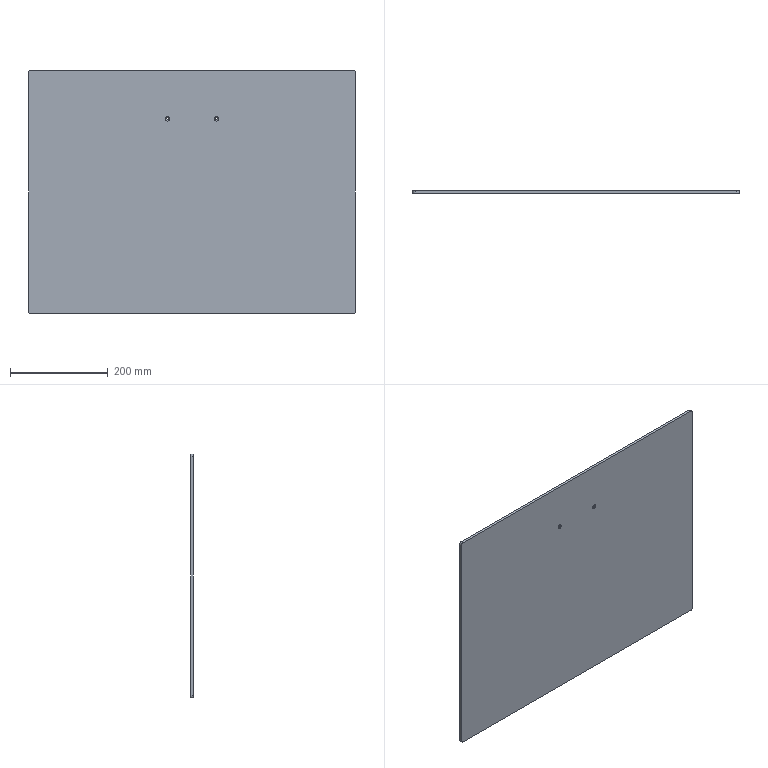Part | NX | features solid 2 | 1 solid | 18 faces | box 670 x 5 x 500 mm | volume 1674617 mm3 | cylinder 8 | plane 6 | cone 4 | commonest cylinder face diameters 5 x4 10 x4
STEP:
#1=CARTESIAN_POINT('',(1510.5,-650.,1045.));
#2=VERTEX_POINT('',#1);
#3=CARTESIAN_POINT('',(1512.5,-648.,1045.));
#4=VERTEX_POINT('',#3);
#5=CARTESIAN_POINT('',(1512.5,-648.,1045.));
#6=DIRECTION('',(-0.7071,-0.7071,0.));
#7=VECTOR('',#6,1000.);
#8=LINE('',#5,#7);
#9=EDGE_CURVE('',#2,#4,#8,.F.);
#10=ORIENTED_EDGE('',*,*,#9,.T.);
#11=CARTESIAN_POINT('',(1517.5,-648.,1045.));
#12=VERTEX_POINT('',#11);
#13=CARTESIAN_POINT('',(1515.,-648.,1045.));
#14=DIRECTION('',(0.,-1.,0.));
#15=DIRECTION('',(1.,0.,0.));
#16=AXIS2_PLACEMENT_3D('',#13,#14,#15);
#17=CIRCLE('',#16,2.5);
#18=EDGE_CURVE('',#12,#4,#17,.T.);
#19=ORIENTED_EDGE('',*,*,#18,.F.);
#20=CARTESIAN_POINT('',(1519.5,-650.,1045.));
#21=VERTEX_POINT('',#20);
#22=CARTESIAN_POINT('',(1517.5,-648.,1045.));
#23=DIRECTION('',(0.7071,-0.7071,0.));
#24=VECTOR('',#23,1000.);
#25=LINE('',#22,#24);
#26=EDGE_CURVE('',#12,#21,#25,.T.);
#27=ORIENTED_EDGE('',*,*,#26,.T.);
#28=CARTESIAN_POINT('',(1515.,-650.,1045.));
#29=DIRECTION('',(0.,1.,0.));
#30=DIRECTION('',(1.,0.,0.));
#31=AXIS2_PLACEMENT_3D('',#28,#29,#30);
#32=CIRCLE('',#31,4.5);
#33=EDGE_CURVE('',#2,#21,#32,.T.);
#34=ORIENTED_EDGE('',*,*,#33,.F.);
#35=EDGE_LOOP('',(#10,#19,#27,#34));
#36=FACE_BOUND('',#35,.T.);
#37=CARTESIAN_POINT('',(1515.,-648.,1045.));
#38=DIRECTION('',(0.,-1.,0.));
#39=DIRECTION('',(1.,0.,0.));
#40=AXIS2_PLACEMENT_3D('',#37,#38,#39);
#41=CONICAL_SURFACE('',#40,2.5,0.7854);
#42=ADVANCED_FACE('',(#36),#41,.F.);
#43=CARTESIAN_POINT('',(1610.5,-650.,1045.));
#44=VERTEX_POINT('',#43);
#45=CARTESIAN_POINT('',(1612.5,-648.,1045.));
#46=VERTEX_POINT('',#45);
#47=CARTESIAN_POINT('',(1612.5,-648.,1045.));
#48=DIRECTION('',(-0.7071,-0.7071,0.));
#49=VECTOR('',#48,1000.);
#50=LINE('',#47,#49);
#51=EDGE_CURVE('',#44,#46,#50,.F.);
#52=ORIENTED_EDGE('',*,*,#51,.T.);
#53=CARTESIAN_POINT('',(1617.5,-648.,1045.));
#54=VERTEX_POINT('',#53);
#55=CARTESIAN_POINT('',(1615.,-648.,1045.));
#56=DIRECTION('',(0.,-1.,0.));
#57=DIRECTION('',(1.,0.,0.));
#58=AXIS2_PLACEMENT_3D('',#55,#56,#57);
#59=CIRCLE('',#58,2.5);
#60=EDGE_CURVE('',#54,#46,#59,.T.);
#61=ORIENTED_EDGE('',*,*,#60,.F.);
#62=CARTESIAN_POINT('',(1619.5,-650.,1045.));
#63=VERTEX_POINT('',#62);
#64=CARTESIAN_POINT('',(1617.5,-648.,1045.));
#65=DIRECTION('',(0.7071,-0.7071,0.));
#66=VECTOR('',#65,1000.);
#67=LINE('',#64,#66);
#68=EDGE_CURVE('',#54,#63,#67,.T.);
#69=ORIENTED_EDGE('',*,*,#68,.T.);
#70=CARTESIAN_POINT('',(1615.,-650.,1045.));
#71=DIRECTION('',(0.,1.,0.));
#72=DIRECTION('',(1.,0.,0.));
#73=AXIS2_PLACEMENT_3D('',#70,#71,#72);
#74=CIRCLE('',#73,4.5);
#75=EDGE_CURVE('',#44,#63,#74,.T.);
#76=ORIENTED_EDGE('',*,*,#75,.F.);
#77=EDGE_LOOP('',(#52,#61,#69,#76));
#78=FACE_BOUND('',#77,.T.);
#79=CARTESIAN_POINT('',(1615.,-648.,1045.));
#80=DIRECTION('',(0.,-1.,0.));
#81=DIRECTION('',(1.,0.,0.));
#82=AXIS2_PLACEMENT_3D('',#79,#80,#81);
#83=CONICAL_SURFACE('',#82,2.5,0.7854);
#84=ADVANCED_FACE('',(#78),#83,.F.);
#85=CARTESIAN_POINT('',(1517.5,-645.,1045.));
#86=VERTEX_POINT('',#85);
#87=CARTESIAN_POINT('',(1517.5,-1481.017,1045.));
#88=DIRECTION('',(0.,1.,0.));
#89=VECTOR('',#88,1000.);
#90=LINE('',#87,#89);
#91=EDGE_CURVE('',#86,#12,#90,.F.);
#92=ORIENTED_EDGE('',*,*,#91,.T.);
#93=ORIENTED_EDGE('',*,*,#18,.T.);
#94=CARTESIAN_POINT('',(1512.5,-645.,1045.));
#95=VERTEX_POINT('',#94);
#96=CARTESIAN_POINT('',(1512.5,-1481.017,1045.));
#97=DIRECTION('',(0.,1.,0.));
#98=VECTOR('',#97,1000.);
#99=LINE('',#96,#98);
#100=EDGE_CURVE('',#4,#95,#99,.T.);
#101=ORIENTED_EDGE('',*,*,#100,.T.);
#102=CARTESIAN_POINT('',(1515.,-645.,1045.));
#103=DIRECTION('',(0.,1.,0.));
#104=DIRECTION('',(-1.,0.,0.));
#105=AXIS2_PLACEMENT_3D('',#102,#103,#104);
#106=CIRCLE('',#105,2.5);
#107=EDGE_CURVE('',#95,#86,#106,.T.);
#108=ORIENTED_EDGE('',*,*,#107,.T.);
#109=EDGE_LOOP('',(#92,#93,#101,#108));
#110=FACE_BOUND('',#109,.T.);
#111=CARTESIAN_POINT('',(1515.,-1481.017,1045.));
#112=DIRECTION('',(0.,1.,0.));
#113=DIRECTION('',(-1.,0.,0.));
#114=AXIS2_PLACEMENT_3D('',#111,#112,#113);
#115=CYLINDRICAL_SURFACE('',#114,2.5);
#116=ADVANCED_FACE('',(#110),#115,.F.);
#117=CARTESIAN_POINT('',(1617.5,-645.,1045.));
#118=VERTEX_POINT('',#117);
#119=CARTESIAN_POINT('',(1617.5,-1481.017,1045.));
#120=DIRECTION('',(0.,1.,0.));
#121=VECTOR('',#120,1000.);
#122=LINE('',#119,#121);
#123=EDGE_CURVE('',#118,#54,#122,.F.);
#124=ORIENTED_EDGE('',*,*,#123,.T.);
#125=ORIENTED_EDGE('',*,*,#60,.T.);
#126=CARTESIAN_POINT('',(1612.5,-645.,1045.));
#127=VERTEX_POINT('',#126);
#128=CARTESIAN_POINT('',(1612.5,-1481.017,1045.));
#129=DIRECTION('',(0.,1.,0.));
#130=VECTOR('',#129,1000.);
#131=LINE('',#128,#130);
#132=EDGE_CURVE('',#46,#127,#131,.T.);
#133=ORIENTED_EDGE('',*,*,#132,.T.);
#134=CARTESIAN_POINT('',(1615.,-645.,1045.));
#135=DIRECTION('',(0.,1.,0.));
#136=DIRECTION('',(-1.,0.,0.));
#137=AXIS2_PLACEMENT_3D('',#134,#135,#136);
#138=CIRCLE('',#137,2.5);
#139=EDGE_CURVE('',#127,#118,#138,.T.);
#140=ORIENTED_EDGE('',*,*,#139,.T.);
#141=EDGE_LOOP('',(#124,#125,#133,#140));
#142=FACE_BOUND('',#141,.T.);
#143=CARTESIAN_POINT('',(1615.,-1481.017,1045.));
#144=DIRECTION('',(0.,1.,0.));
#145=DIRECTION('',(-1.,0.,0.));
#146=AXIS2_PLACEMENT_3D('',#143,#144,#145);
#147=CYLINDRICAL_SURFACE('',#146,2.5);
#148=ADVANCED_FACE('',(#142),#147,.F.);
#149=CARTESIAN_POINT('',(1235.,-645.,645.));
#150=VERTEX_POINT('',#149);
#151=CARTESIAN_POINT('',(1230.,-645.,650.));
#152=VERTEX_POINT('',#151);
#153=CARTESIAN_POINT('',(1235.,-645.,650.));
#154=DIRECTION('',(0.,1.,0.));
#155=DIRECTION('',(1.,0.,0.));
#156=AXIS2_PLACEMENT_3D('',#153,#154,#155);
#157=CIRCLE('',#156,5.);
#158=EDGE_CURVE('',#150,#152,#157,.T.);
#159=ORIENTED_EDGE('',*,*,#158,.F.);
#160=CARTESIAN_POINT('',(1235.,-650.,645.));
#161=VERTEX_POINT('',#160);
#162=CARTESIAN_POINT('',(1235.,-645.,645.));
#163=DIRECTION('',(0.,1.,0.));
#164=VECTOR('',#163,1000.);
#165=LINE('',#162,#164);
#166=EDGE_CURVE('',#161,#150,#165,.T.);
#167=ORIENTED_EDGE('',*,*,#166,.F.);
#168=CARTESIAN_POINT('',(1230.,-650.,650.));
#169=VERTEX_POINT('',#168);
#170=CARTESIAN_POINT('',(1235.,-650.,650.));
#171=DIRECTION('',(0.,-1.,0.));
#172=DIRECTION('',(1.,0.,0.));
#173=AXIS2_PLACEMENT_3D('',#170,#171,#172);
#174=CIRCLE('',#173,5.);
#175=EDGE_CURVE('',#169,#161,#174,.T.);
#176=ORIENTED_EDGE('',*,*,#175,.F.);
#177=CARTESIAN_POINT('',(1230.,-645.,650.));
#178=DIRECTION('',(0.,-1.,0.));
#179=VECTOR('',#178,1000.);
#180=LINE('',#177,#179);
#181=EDGE_CURVE('',#152,#169,#180,.T.);
#182=ORIENTED_EDGE('',*,*,#181,.F.);
#183=EDGE_LOOP('',(#159,#167,#176,#182));
#184=FACE_BOUND('',#183,.T.);
#185=CARTESIAN_POINT('',(1235.,-645.,650.));
#186=DIRECTION('',(0.,-1.,0.));
#187=DIRECTION('',(1.,0.,0.));
#188=AXIS2_PLACEMENT_3D('',#185,#186,#187);
#189=CYLINDRICAL_SURFACE('',#188,5.);
#190=ADVANCED_FACE('',(#184),#189,.T.);
#191=CARTESIAN_POINT('',(1230.,-645.,1140.));
#192=VERTEX_POINT('',#191);
#193=CARTESIAN_POINT('',(1235.,-645.,1145.));
#194=VERTEX_POINT('',#193);
#195=CARTESIAN_POINT('',(1235.,-645.,1140.));
#196=DIRECTION('',(0.,1.,0.));
#197=DIRECTION('',(1.,0.,0.));
#198=AXIS2_PLACEMENT_3D('',#195,#196,#197);
#199=CIRCLE('',#198,5.);
#200=EDGE_CURVE('',#192,#194,#199,.T.);
#201=ORIENTED_EDGE('',*,*,#200,.F.);
#202=CARTESIAN_POINT('',(1230.,-650.,1140.));
#203=VERTEX_POINT('',#202);
#204=CARTESIAN_POINT('',(1230.,-645.,1140.));
#205=DIRECTION('',(0.,1.,0.));
#206=VECTOR('',#205,1000.);
#207=LINE('',#204,#206);
#208=EDGE_CURVE('',#203,#192,#207,.T.);
#209=ORIENTED_EDGE('',*,*,#208,.F.);
#210=CARTESIAN_POINT('',(1235.,-650.,1145.));
#211=VERTEX_POINT('',#210);
#212=CARTESIAN_POINT('',(1235.,-650.,1140.));
#213=DIRECTION('',(0.,-1.,0.));
#214=DIRECTION('',(1.,0.,0.));
#215=AXIS2_PLACEMENT_3D('',#212,#213,#214);
#216=CIRCLE('',#215,5.);
#217=EDGE_CURVE('',#211,#203,#216,.T.);
#218=ORIENTED_EDGE('',*,*,#217,.F.);
#219=CARTESIAN_POINT('',(1235.,-645.,1145.));
#220=DIRECTION('',(0.,-1.,0.));
#221=VECTOR('',#220,1000.);
#222=LINE('',#219,#221);
#223=EDGE_CURVE('',#194,#211,#222,.T.);
#224=ORIENTED_EDGE('',*,*,#223,.F.);
#225=EDGE_LOOP('',(#201,#209,#218,#224));
#226=FACE_BOUND('',#225,.T.);
#227=CARTESIAN_POINT('',(1235.,-645.,1140.));
#228=DIRECTION('',(0.,-1.,0.));
#229=DIRECTION('',(1.,0.,0.));
#230=AXIS2_PLACEMENT_3D('',#227,#228,#229);
#231=CYLINDRICAL_SURFACE('',#230,5.);
#232=ADVANCED_FACE('',(#226),#231,.T.);
#233=CARTESIAN_POINT('',(1895.,-645.,1145.));
#234=VERTEX_POINT('',#233);
#235=CARTESIAN_POINT('',(1900.,-645.,1140.));
#236=VERTEX_POINT('',#235);
#237=CARTESIAN_POINT('',(1895.,-645.,1140.));
#238=DIRECTION('',(0.,1.,0.));
#239=DIRECTION('',(1.,0.,0.));
#240=AXIS2_PLACEMENT_3D('',#237,#238,#239);
#241=CIRCLE('',#240,5.);
#242=EDGE_CURVE('',#234,#236,#241,.T.);
#243=ORIENTED_EDGE('',*,*,#242,.F.);
#244=CARTESIAN_POINT('',(1895.,-650.,1145.));
#245=VERTEX_POINT('',#244);
#246=CARTESIAN_POINT('',(1895.,-645.,1145.));
#247=DIRECTION('',(0.,1.,0.));
#248=VECTOR('',#247,1000.);
#249=LINE('',#246,#248);
#250=EDGE_CURVE('',#245,#234,#249,.T.);
#251=ORIENTED_EDGE('',*,*,#250,.F.);
#252=CARTESIAN_POINT('',(1900.,-650.,1140.));
#253=VERTEX_POINT('',#252);
#254=CARTESIAN_POINT('',(1895.,-650.,1140.));
#255=DIRECTION('',(0.,-1.,0.));
#256=DIRECTION('',(1.,0.,0.));
#257=AXIS2_PLACEMENT_3D('',#254,#255,#256);
#258=CIRCLE('',#257,5.);
#259=EDGE_CURVE('',#253,#245,#258,.T.);
#260=ORIENTED_EDGE('',*,*,#259,.F.);
#261=CARTESIAN_POINT('',(1900.,-645.,1140.));
#262=DIRECTION('',(0.,-1.,0.));
#263=VECTOR('',#262,1000.);
#264=LINE('',#261,#263);
#265=EDGE_CURVE('',#236,#253,#264,.T.);
#266=ORIENTED_EDGE('',*,*,#265,.F.);
#267=EDGE_LOOP('',(#243,#251,#260,#266));
#268=FACE_BOUND('',#267,.T.);
#269=CARTESIAN_POINT('',(1895.,-645.,1140.));
#270=DIRECTION('',(0.,-1.,0.));
#271=DIRECTION('',(1.,0.,0.));
#272=AXIS2_PLACEMENT_3D('',#269,#270,#271);
#273=CYLINDRICAL_SURFACE('',#272,5.);
#274=ADVANCED_FACE('',(#268),#273,.T.);
#275=CARTESIAN_POINT('',(1900.,-645.,650.));
#276=VERTEX_POINT('',#275);
#277=CARTESIAN_POINT('',(1895.,-645.,645.));
#278=VERTEX_POINT('',#277);
#279=CARTESIAN_POINT('',(1895.,-645.,650.));
#280=DIRECTION('',(0.,1.,0.));
#281=DIRECTION('',(1.,0.,0.));
#282=AXIS2_PLACEMENT_3D('',#279,#280,#281);
#283=CIRCLE('',#282,5.);
#284=EDGE_CURVE('',#276,#278,#283,.T.);
#285=ORIENTED_EDGE('',*,*,#284,.F.);
#286=CARTESIAN_POINT('',(1900.,-650.,650.));
#287=VERTEX_POINT('',#286);
#288=CARTESIAN_POINT('',(1900.,-645.,650.));
#289=DIRECTION('',(0.,1.,0.));
#290=VECTOR('',#289,1000.);
#291=LINE('',#288,#290);
#292=EDGE_CURVE('',#287,#276,#291,.T.);
#293=ORIENTED_EDGE('',*,*,#292,.F.);
#294=CARTESIAN_POINT('',(1895.,-650.,645.));
#295=VERTEX_POINT('',#294);
#296=CARTESIAN_POINT('',(1895.,-650.,650.));
#297=DIRECTION('',(0.,-1.,0.));
#298=DIRECTION('',(1.,0.,0.));
#299=AXIS2_PLACEMENT_3D('',#296,#297,#298);
#300=CIRCLE('',#299,5.);
#301=EDGE_CURVE('',#295,#287,#300,.T.);
#302=ORIENTED_EDGE('',*,*,#301,.F.);
#303=CARTESIAN_POINT('',(1895.,-645.,645.));
#304=DIRECTION('',(0.,-1.,0.));
#305=VECTOR('',#304,1000.);
#306=LINE('',#303,#305);
#307=EDGE_CURVE('',#278,#295,#306,.T.);
#308=ORIENTED_EDGE('',*,*,#307,.F.);
#309=EDGE_LOOP('',(#285,#293,#302,#308));
#310=FACE_BOUND('',#309,.T.);
#311=CARTESIAN_POINT('',(1895.,-645.,650.));
#312=DIRECTION('',(0.,-1.,0.));
#313=DIRECTION('',(1.,0.,0.));
#314=AXIS2_PLACEMENT_3D('',#311,#312,#313);
#315=CYLINDRICAL_SURFACE('',#314,5.);
#316=ADVANCED_FACE('',(#310),#315,.T.);
#317=CARTESIAN_POINT('',(1515.,-650.,1045.));
#318=DIRECTION('',(0.,1.,0.));
#319=DIRECTION('',(1.,0.,0.));
#320=AXIS2_PLACEMENT_3D('',#317,#318,#319);
#321=CIRCLE('',#320,4.5);
#322=EDGE_CURVE('',#21,#2,#321,.T.);
#323=ORIENTED_EDGE('',*,*,#322,.T.);
#324=ORIENTED_EDGE('',*,*,#33,.T.);
#325=EDGE_LOOP('',(#323,#324));
#326=FACE_BOUND('',#325,.T.);
#327=CARTESIAN_POINT('',(1615.,-650.,1045.));
#328=DIRECTION('',(0.,1.,0.));
#329=DIRECTION('',(1.,0.,0.));
#330=AXIS2_PLACEMENT_3D('',#327,#328,#329);
#331=CIRCLE('',#330,4.5);
#332=EDGE_CURVE('',#63,#44,#331,.T.);
#333=ORIENTED_EDGE('',*,*,#332,.T.);
#334=ORIENTED_EDGE('',*,*,#75,.T.);
#335=EDGE_LOOP('',(#333,#334));
#336=FACE_BOUND('',#335,.T.);
#337=CARTESIAN_POINT('',(1230.,-650.,1145.));
#338=DIRECTION('',(0.,0.,-1.));
#339=VECTOR('',#338,1000.);
#340=LINE('',#337,#339);
#341=EDGE_CURVE('',#203,#169,#340,.T.);
#342=ORIENTED_EDGE('',*,*,#341,.T.);
#343=ORIENTED_EDGE('',*,*,#175,.T.);
#344=CARTESIAN_POINT('',(1230.,-650.,645.));
#345=DIRECTION('',(1.,0.,0.));
#346=VECTOR('',#345,1000.);
#347=LINE('',#344,#346);
#348=EDGE_CURVE('',#161,#295,#347,.T.);
#349=ORIENTED_EDGE('',*,*,#348,.T.);
#350=ORIENTED_EDGE('',*,*,#301,.T.);
#351=CARTESIAN_POINT('',(1900.,-650.,645.));
#352=DIRECTION('',(0.,0.,1.));
#353=VECTOR('',#352,1000.);
#354=LINE('',#351,#353);
#355=EDGE_CURVE('',#287,#253,#354,.T.);
#356=ORIENTED_EDGE('',*,*,#355,.T.);
#357=ORIENTED_EDGE('',*,*,#259,.T.);
#358=CARTESIAN_POINT('',(1900.,-650.,1145.));
#359=DIRECTION('',(-1.,0.,0.));
#360=VECTOR('',#359,1000.);
#361=LINE('',#358,#360);
#362=EDGE_CURVE('',#245,#211,#361,.T.);
#363=ORIENTED_EDGE('',*,*,#362,.T.);
#364=ORIENTED_EDGE('',*,*,#217,.T.);
#365=EDGE_LOOP('',(#342,#343,#349,#350,#356,#357,#363,#364));
#366=FACE_BOUND('',#365,.T.);
#367=CARTESIAN_POINT('',(1565.,-650.,895.));
#368=DIRECTION('',(0.,-1.,0.));
#369=DIRECTION('',(-1.,0.,0.));
#370=AXIS2_PLACEMENT_3D('',#367,#368,#369);
#371=PLANE('',#370);
#372=ADVANCED_FACE('',(#326,#336,#366),#371,.T.);
#373=ORIENTED_EDGE('',*,*,#139,.F.);
#374=CARTESIAN_POINT('',(1615.,-645.,1045.));
#375=DIRECTION('',(0.,1.,0.));
#376=DIRECTION('',(-1.,0.,0.));
#377=AXIS2_PLACEMENT_3D('',#374,#375,#376);
#378=CIRCLE('',#377,2.5);
#379=EDGE_CURVE('',#118,#127,#378,.T.);
#380=ORIENTED_EDGE('',*,*,#379,.F.);
#381=EDGE_LOOP('',(#373,#380));
#382=FACE_BOUND('',#381,.T.);
#383=ORIENTED_EDGE('',*,*,#107,.F.);
#384=CARTESIAN_POINT('',(1515.,-645.,1045.));
#385=DIRECTION('',(0.,1.,0.));
#386=DIRECTION('',(-1.,0.,0.));
#387=AXIS2_PLACEMENT_3D('',#384,#385,#386);
#388=CIRCLE('',#387,2.5);
#389=EDGE_CURVE('',#86,#95,#388,.T.);
#390=ORIENTED_EDGE('',*,*,#389,.F.);
#391=EDGE_LOOP('',(#383,#390));
#392=FACE_BOUND('',#391,.T.);
#393=CARTESIAN_POINT('',(1230.,-645.,645.));
#394=DIRECTION('',(1.,0.,0.));
#395=VECTOR('',#394,1000.);
#396=LINE('',#393,#395);
#397=EDGE_CURVE('',#150,#278,#396,.T.);
#398=ORIENTED_EDGE('',*,*,#397,.F.);
#399=ORIENTED_EDGE('',*,*,#158,.T.);
#400=CARTESIAN_POINT('',(1230.,-645.,1145.));
#401=DIRECTION('',(0.,0.,-1.));
#402=VECTOR('',#401,1000.);
#403=LINE('',#400,#402);
#404=EDGE_CURVE('',#192,#152,#403,.T.);
#405=ORIENTED_EDGE('',*,*,#404,.F.);
#406=ORIENTED_EDGE('',*,*,#200,.T.);
#407=CARTESIAN_POINT('',(1900.,-645.,1145.));
#408=DIRECTION('',(-1.,0.,0.));
#409=VECTOR('',#408,1000.);
#410=LINE('',#407,#409);
#411=EDGE_CURVE('',#234,#194,#410,.T.);
#412=ORIENTED_EDGE('',*,*,#411,.F.);
#413=ORIENTED_EDGE('',*,*,#242,.T.);
#414=CARTESIAN_POINT('',(1900.,-645.,645.));
#415=DIRECTION('',(0.,0.,1.));
#416=VECTOR('',#415,1000.);
#417=LINE('',#414,#416);
#418=EDGE_CURVE('',#276,#236,#417,.T.);
#419=ORIENTED_EDGE('',*,*,#418,.F.);
#420=ORIENTED_EDGE('',*,*,#284,.T.);
#421=EDGE_LOOP('',(#398,#399,#405,#406,#412,#413,#419,#420));
#422=FACE_BOUND('',#421,.T.);
#423=CARTESIAN_POINT('',(1565.,-645.,895.));
#424=DIRECTION('',(0.,-1.,0.));
#425=DIRECTION('',(-1.,0.,0.));
#426=AXIS2_PLACEMENT_3D('',#423,#424,#425);
#427=PLANE('',#426);
#428=ADVANCED_FACE('',(#382,#392,#422),#427,.F.);
#429=ORIENTED_EDGE('',*,*,#411,.T.);
#430=ORIENTED_EDGE('',*,*,#223,.T.);
#431=ORIENTED_EDGE('',*,*,#362,.F.);
#432=ORIENTED_EDGE('',*,*,#250,.T.);
#433=EDGE_LOOP('',(#429,#430,#431,#432));
#434=FACE_BOUND('',#433,.T.);
#435=CARTESIAN_POINT('',(1900.,-645.,1145.));
#436=DIRECTION('',(0.,0.,1.));
#437=DIRECTION('',(1.,0.,0.));
#438=AXIS2_PLACEMENT_3D('',#435,#436,#437);
#439=PLANE('',#438);
#440=ADVANCED_FACE('',(#434),#439,.T.);
#441=ORIENTED_EDGE('',*,*,#418,.T.);
#442=ORIENTED_EDGE('',*,*,#265,.T.);
#443=ORIENTED_EDGE('',*,*,#355,.F.);
#444=ORIENTED_EDGE('',*,*,#292,.T.);
#445=EDGE_LOOP('',(#441,#442,#443,#444));
#446=FACE_BOUND('',#445,.T.);
#447=CARTESIAN_POINT('',(1900.,-645.,645.));
#448=DIRECTION('',(1.,0.,0.));
#449=DIRECTION('',(0.,0.,1.));
#450=AXIS2_PLACEMENT_3D('',#447,#448,#449);
#451=PLANE('',#450);
#452=ADVANCED_FACE('',(#446),#451,.T.);
#453=ORIENTED_EDGE('',*,*,#348,.F.);
#454=ORIENTED_EDGE('',*,*,#166,.T.);
#455=ORIENTED_EDGE('',*,*,#397,.T.);
#456=ORIENTED_EDGE('',*,*,#307,.T.);
#457=EDGE_LOOP('',(#453,#454,#455,#456));
#458=FACE_BOUND('',#457,.T.);
#459=CARTESIAN_POINT('',(1230.,-645.,645.));
#460=DIRECTION('',(0.,0.,-1.));
#461=DIRECTION('',(0.,-1.,0.));
#462=AXIS2_PLACEMENT_3D('',#459,#460,#461);
#463=PLANE('',#462);
#464=ADVANCED_FACE('',(#458),#463,.T.);
#465=ORIENTED_EDGE('',*,*,#404,.T.);
#466=ORIENTED_EDGE('',*,*,#181,.T.);
#467=ORIENTED_EDGE('',*,*,#341,.F.);
#468=ORIENTED_EDGE('',*,*,#208,.T.);
#469=EDGE_LOOP('',(#465,#466,#467,#468));
#470=FACE_BOUND('',#469,.T.);
#471=CARTESIAN_POINT('',(1230.,-645.,1145.));
#472=DIRECTION('',(-1.,0.,0.));
#473=DIRECTION('',(0.,0.,1.));
#474=AXIS2_PLACEMENT_3D('',#471,#472,#473);
#475=PLANE('',#474);
#476=ADVANCED_FACE('',(#470),#475,.T.);
#477=CARTESIAN_POINT('',(1615.,-648.,1045.));
#478=DIRECTION('',(0.,-1.,0.));
#479=DIRECTION('',(1.,0.,0.));
#480=AXIS2_PLACEMENT_3D('',#477,#478,#479);
#481=CIRCLE('',#480,2.5);
#482=EDGE_CURVE('',#46,#54,#481,.T.);
#483=ORIENTED_EDGE('',*,*,#482,.T.);
#484=ORIENTED_EDGE('',*,*,#123,.F.);
#485=ORIENTED_EDGE('',*,*,#379,.T.);
#486=ORIENTED_EDGE('',*,*,#132,.F.);
#487=EDGE_LOOP('',(#483,#484,#485,#486));
#488=FACE_BOUND('',#487,.T.);
#489=CARTESIAN_POINT('',(1615.,-1481.017,1045.));
#490=DIRECTION('',(0.,1.,0.));
#491=DIRECTION('',(-1.,0.,0.));
#492=AXIS2_PLACEMENT_3D('',#489,#490,#491);
#493=CYLINDRICAL_SURFACE('',#492,2.5);
#494=ADVANCED_FACE('',(#488),#493,.F.);
#495=CARTESIAN_POINT('',(1515.,-648.,1045.));
#496=DIRECTION('',(0.,-1.,0.));
#497=DIRECTION('',(1.,0.,0.));
#498=AXIS2_PLACEMENT_3D('',#495,#496,#497);
#499=CIRCLE('',#498,2.5);
#500=EDGE_CURVE('',#4,#12,#499,.T.);
#501=ORIENTED_EDGE('',*,*,#500,.T.);
#502=ORIENTED_EDGE('',*,*,#91,.F.);
#503=ORIENTED_EDGE('',*,*,#389,.T.);
#504=ORIENTED_EDGE('',*,*,#100,.F.);
#505=EDGE_LOOP('',(#501,#502,#503,#504));
#506=FACE_BOUND('',#505,.T.);
#507=CARTESIAN_POINT('',(1515.,-1481.017,1045.));
#508=DIRECTION('',(0.,1.,0.));
#509=DIRECTION('',(-1.,0.,0.));
#510=AXIS2_PLACEMENT_3D('',#507,#508,#509);
#511=CYLINDRICAL_SURFACE('',#510,2.5);
#512=ADVANCED_FACE('',(#506),#511,.F.);
#513=ORIENTED_EDGE('',*,*,#482,.F.);
#514=ORIENTED_EDGE('',*,*,#51,.F.);
#515=ORIENTED_EDGE('',*,*,#332,.F.);
#516=ORIENTED_EDGE('',*,*,#68,.F.);
#517=EDGE_LOOP('',(#513,#514,#515,#516));
#518=FACE_BOUND('',#517,.T.);
#519=CARTESIAN_POINT('',(1615.,-648.,1045.));
#520=DIRECTION('',(0.,-1.,0.));
#521=DIRECTION('',(1.,0.,0.));
#522=AXIS2_PLACEMENT_3D('',#519,#520,#521);
#523=CONICAL_SURFACE('',#522,2.5,0.7854);
#524=ADVANCED_FACE('',(#518),#523,.F.);
#525=ORIENTED_EDGE('',*,*,#500,.F.);
#526=ORIENTED_EDGE('',*,*,#9,.F.);
#527=ORIENTED_EDGE('',*,*,#322,.F.);
#528=ORIENTED_EDGE('',*,*,#26,.F.);
#529=EDGE_LOOP('',(#525,#526,#527,#528));
#530=FACE_BOUND('',#529,.T.);
#531=CARTESIAN_POINT('',(1515.,-648.,1045.));
#532=DIRECTION('',(0.,-1.,0.));
#533=DIRECTION('',(1.,0.,0.));
#534=AXIS2_PLACEMENT_3D('',#531,#532,#533);
#535=CONICAL_SURFACE('',#534,2.5,0.7854);
#536=ADVANCED_FACE('',(#530),#535,.F.);
#537=CLOSED_SHELL('',(#42,#84,#116,#148,#190,#232,#274,#316,#372,#428,#440,#452,#464,#476,#494,#512,#524,#536));
#538=MANIFOLD_SOLID_BREP('',#537);
#539=(LENGTH_UNIT()NAMED_UNIT(*)SI_UNIT(.MILLI.,.METRE.));
#540=UNCERTAINTY_MEASURE_WITH_UNIT(LENGTH_MEASURE(0.00001),#539,'','');
#541=(NAMED_UNIT(*)PLANE_ANGLE_UNIT()SI_UNIT($,.RADIAN.));
#542=(NAMED_UNIT(*)SI_UNIT($,.STERADIAN.)SOLID_ANGLE_UNIT());
#543=(GEOMETRIC_REPRESENTATION_CONTEXT(3)GLOBAL_UNCERTAINTY_ASSIGNED_CONTEXT((#540))GLOBAL_UNIT_ASSIGNED_CONTEXT((#539,#541,#542))REPRESENTATION_CONTEXT('',''));
#544=ADVANCED_BREP_SHAPE_REPRESENTATION('',(#538),#543);